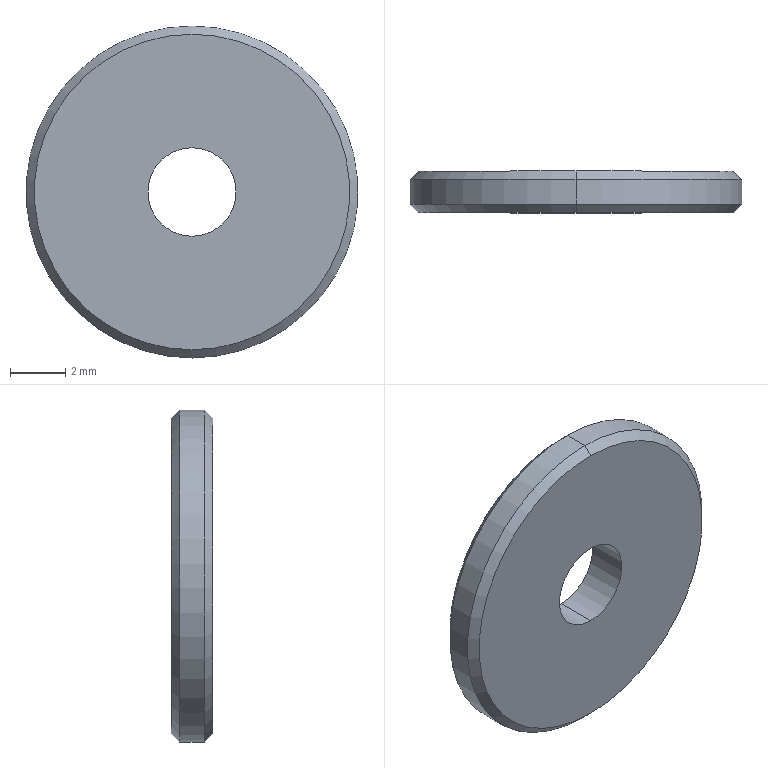Part | SolidWorks | features Chamfer 1, Extrusion 1 | 1 solid | 10 faces | box 12 x 1.5 x 12 mm | volume 154.246 mm3 | cone 4 | cylinder 4 | plane 2 | commonest cylinder face diameters 3.2 x2 12 x2
STEP:
#1=CARTESIAN_POINT('',(0.,1.5,5.7));
#2=VERTEX_POINT('',#1);
#3=CARTESIAN_POINT('',(0.,1.5,-5.7));
#4=VERTEX_POINT('',#3);
#5=CARTESIAN_POINT('',(0.,1.5,0.));
#6=DIRECTION('',(0.,1.,0.));
#7=DIRECTION('',(0.,0.,1.));
#8=AXIS2_PLACEMENT_3D('',#5,#6,#7);
#9=CIRCLE('',#8,5.7);
#10=EDGE_CURVE('',#2,#4,#9,.T.);
#11=ORIENTED_EDGE('',*,*,#10,.F.);
#12=CARTESIAN_POINT('',(0.,1.2,6.));
#13=VERTEX_POINT('',#12);
#14=CARTESIAN_POINT('',(0.,1.5,5.7));
#15=DIRECTION('',(0.,-0.7071,0.7071));
#16=VECTOR('',#15,1000.);
#17=LINE('',#14,#16);
#18=EDGE_CURVE('',#2,#13,#17,.T.);
#19=ORIENTED_EDGE('',*,*,#18,.T.);
#20=CARTESIAN_POINT('',(0.,1.2,-6.));
#21=VERTEX_POINT('',#20);
#22=CARTESIAN_POINT('',(0.,1.2,0.));
#23=DIRECTION('',(0.,-1.,0.));
#24=DIRECTION('',(0.,0.,1.));
#25=AXIS2_PLACEMENT_3D('',#22,#23,#24);
#26=CIRCLE('',#25,6.);
#27=EDGE_CURVE('',#21,#13,#26,.T.);
#28=ORIENTED_EDGE('',*,*,#27,.F.);
#29=CARTESIAN_POINT('',(0.,1.5,-5.7));
#30=DIRECTION('',(0.,-0.7071,-0.7071));
#31=VECTOR('',#30,1000.);
#32=LINE('',#29,#31);
#33=EDGE_CURVE('',#4,#21,#32,.T.);
#34=ORIENTED_EDGE('',*,*,#33,.F.);
#35=EDGE_LOOP('',(#11,#19,#28,#34));
#36=FACE_OUTER_BOUND('',#35,.T.);
#37=CARTESIAN_POINT('',(0.,1.5,0.));
#38=DIRECTION('',(0.,-1.,0.));
#39=DIRECTION('',(0.,0.,-1.));
#40=AXIS2_PLACEMENT_3D('',#37,#38,#39);
#41=CONICAL_SURFACE('',#40,5.7,0.7854);
#42=ADVANCED_FACE('',(#36),#41,.T.);
#43=CARTESIAN_POINT('',(0.,0.,-5.7));
#44=VERTEX_POINT('',#43);
#45=CARTESIAN_POINT('',(0.,0.,5.7));
#46=VERTEX_POINT('',#45);
#47=CARTESIAN_POINT('',(0.,0.,0.));
#48=DIRECTION('',(0.,-1.,0.));
#49=DIRECTION('',(0.,0.,1.));
#50=AXIS2_PLACEMENT_3D('',#47,#48,#49);
#51=CIRCLE('',#50,5.7);
#52=EDGE_CURVE('',#44,#46,#51,.T.);
#53=ORIENTED_EDGE('',*,*,#52,.F.);
#54=CARTESIAN_POINT('',(0.,0.3,-6.));
#55=VERTEX_POINT('',#54);
#56=CARTESIAN_POINT('',(0.,0.3,-6.));
#57=DIRECTION('',(0.,0.7071,-0.7071));
#58=VECTOR('',#57,1000.);
#59=LINE('',#56,#58);
#60=EDGE_CURVE('',#44,#55,#59,.T.);
#61=ORIENTED_EDGE('',*,*,#60,.T.);
#62=CARTESIAN_POINT('',(0.,0.3,6.));
#63=VERTEX_POINT('',#62);
#64=CARTESIAN_POINT('',(0.,0.3,0.));
#65=DIRECTION('',(0.,1.,0.));
#66=DIRECTION('',(0.,0.,1.));
#67=AXIS2_PLACEMENT_3D('',#64,#65,#66);
#68=CIRCLE('',#67,6.);
#69=EDGE_CURVE('',#63,#55,#68,.T.);
#70=ORIENTED_EDGE('',*,*,#69,.F.);
#71=CARTESIAN_POINT('',(0.,0.3,6.));
#72=DIRECTION('',(0.,0.7071,0.7071));
#73=VECTOR('',#72,1000.);
#74=LINE('',#71,#73);
#75=EDGE_CURVE('',#46,#63,#74,.T.);
#76=ORIENTED_EDGE('',*,*,#75,.F.);
#77=EDGE_LOOP('',(#53,#61,#70,#76));
#78=FACE_OUTER_BOUND('',#77,.T.);
#79=CARTESIAN_POINT('',(0.,0.3,0.));
#80=DIRECTION('',(0.,1.,0.));
#81=DIRECTION('',(0.,0.,1.));
#82=AXIS2_PLACEMENT_3D('',#79,#80,#81);
#83=CONICAL_SURFACE('',#82,6.,0.7854);
#84=ADVANCED_FACE('',(#78),#83,.T.);
#85=CARTESIAN_POINT('',(0.,1.5,-1.6));
#86=VERTEX_POINT('',#85);
#87=CARTESIAN_POINT('',(0.,1.5,1.6));
#88=VERTEX_POINT('',#87);
#89=CARTESIAN_POINT('',(0.,1.5,0.));
#90=DIRECTION('',(0.,1.,0.));
#91=DIRECTION('',(0.,0.,1.));
#92=AXIS2_PLACEMENT_3D('',#89,#90,#91);
#93=CIRCLE('',#92,1.6);
#94=EDGE_CURVE('',#86,#88,#93,.T.);
#95=ORIENTED_EDGE('',*,*,#94,.T.);
#96=CARTESIAN_POINT('',(0.,0.,1.6));
#97=VERTEX_POINT('',#96);
#98=CARTESIAN_POINT('',(0.,1.5,1.6));
#99=DIRECTION('',(0.,-1.,0.));
#100=VECTOR('',#99,1000.);
#101=LINE('',#98,#100);
#102=EDGE_CURVE('',#88,#97,#101,.T.);
#103=ORIENTED_EDGE('',*,*,#102,.T.);
#104=CARTESIAN_POINT('',(0.,0.,-1.6));
#105=VERTEX_POINT('',#104);
#106=CARTESIAN_POINT('',(0.,0.,0.));
#107=DIRECTION('',(0.,1.,0.));
#108=DIRECTION('',(0.,0.,1.));
#109=AXIS2_PLACEMENT_3D('',#106,#107,#108);
#110=CIRCLE('',#109,1.6);
#111=EDGE_CURVE('',#105,#97,#110,.T.);
#112=ORIENTED_EDGE('',*,*,#111,.F.);
#113=CARTESIAN_POINT('',(0.,1.5,-1.6));
#114=DIRECTION('',(0.,-1.,0.));
#115=VECTOR('',#114,1000.);
#116=LINE('',#113,#115);
#117=EDGE_CURVE('',#86,#105,#116,.T.);
#118=ORIENTED_EDGE('',*,*,#117,.F.);
#119=EDGE_LOOP('',(#95,#103,#112,#118));
#120=FACE_OUTER_BOUND('',#119,.T.);
#121=CARTESIAN_POINT('',(0.,1.5,0.));
#122=DIRECTION('',(0.,-1.,0.));
#123=DIRECTION('',(0.,0.,-1.));
#124=AXIS2_PLACEMENT_3D('',#121,#122,#123);
#125=CYLINDRICAL_SURFACE('',#124,1.6);
#126=ADVANCED_FACE('',(#120),#125,.F.);
#127=ORIENTED_EDGE('',*,*,#27,.T.);
#128=CARTESIAN_POINT('',(0.,1.5,6.));
#129=DIRECTION('',(0.,-1.,0.));
#130=VECTOR('',#129,1000.);
#131=LINE('',#128,#130);
#132=EDGE_CURVE('',#13,#63,#131,.T.);
#133=ORIENTED_EDGE('',*,*,#132,.T.);
#134=ORIENTED_EDGE('',*,*,#69,.T.);
#135=CARTESIAN_POINT('',(0.,1.5,-6.));
#136=DIRECTION('',(0.,-1.,0.));
#137=VECTOR('',#136,1000.);
#138=LINE('',#135,#137);
#139=EDGE_CURVE('',#21,#55,#138,.T.);
#140=ORIENTED_EDGE('',*,*,#139,.F.);
#141=EDGE_LOOP('',(#127,#133,#134,#140));
#142=FACE_OUTER_BOUND('',#141,.T.);
#143=CARTESIAN_POINT('',(0.,1.5,0.));
#144=DIRECTION('',(0.,-1.,0.));
#145=DIRECTION('',(0.,0.,-1.));
#146=AXIS2_PLACEMENT_3D('',#143,#144,#145);
#147=CYLINDRICAL_SURFACE('',#146,6.);
#148=ADVANCED_FACE('',(#142),#147,.T.);
#149=CARTESIAN_POINT('',(0.,1.5,0.));
#150=DIRECTION('',(0.,1.,0.));
#151=DIRECTION('',(0.,0.,1.));
#152=AXIS2_PLACEMENT_3D('',#149,#150,#151);
#153=CIRCLE('',#152,5.7);
#154=EDGE_CURVE('',#4,#2,#153,.T.);
#155=ORIENTED_EDGE('',*,*,#154,.T.);
#156=ORIENTED_EDGE('',*,*,#10,.T.);
#157=EDGE_LOOP('',(#155,#156));
#158=FACE_OUTER_BOUND('',#157,.T.);
#159=ORIENTED_EDGE('',*,*,#94,.F.);
#160=CARTESIAN_POINT('',(0.,1.5,0.));
#161=DIRECTION('',(0.,1.,0.));
#162=DIRECTION('',(0.,0.,1.));
#163=AXIS2_PLACEMENT_3D('',#160,#161,#162);
#164=CIRCLE('',#163,1.6);
#165=EDGE_CURVE('',#88,#86,#164,.T.);
#166=ORIENTED_EDGE('',*,*,#165,.F.);
#167=EDGE_LOOP('',(#159,#166));
#168=FACE_BOUND('',#167,.T.);
#169=CARTESIAN_POINT('',(0.,1.5,0.));
#170=DIRECTION('',(0.,1.,0.));
#171=DIRECTION('',(0.,0.,1.));
#172=AXIS2_PLACEMENT_3D('',#169,#170,#171);
#173=PLANE('',#172);
#174=ADVANCED_FACE('',(#158,#168),#173,.T.);
#175=CARTESIAN_POINT('',(0.,0.,0.));
#176=DIRECTION('',(0.,-1.,0.));
#177=DIRECTION('',(0.,0.,1.));
#178=AXIS2_PLACEMENT_3D('',#175,#176,#177);
#179=CIRCLE('',#178,5.7);
#180=EDGE_CURVE('',#46,#44,#179,.T.);
#181=ORIENTED_EDGE('',*,*,#180,.T.);
#182=ORIENTED_EDGE('',*,*,#52,.T.);
#183=EDGE_LOOP('',(#181,#182));
#184=FACE_OUTER_BOUND('',#183,.T.);
#185=ORIENTED_EDGE('',*,*,#111,.T.);
#186=CARTESIAN_POINT('',(0.,0.,0.));
#187=DIRECTION('',(0.,1.,0.));
#188=DIRECTION('',(0.,0.,1.));
#189=AXIS2_PLACEMENT_3D('',#186,#187,#188);
#190=CIRCLE('',#189,1.6);
#191=EDGE_CURVE('',#97,#105,#190,.T.);
#192=ORIENTED_EDGE('',*,*,#191,.T.);
#193=EDGE_LOOP('',(#185,#192));
#194=FACE_BOUND('',#193,.T.);
#195=CARTESIAN_POINT('',(0.,0.,0.));
#196=DIRECTION('',(0.,1.,0.));
#197=DIRECTION('',(0.,0.,1.));
#198=AXIS2_PLACEMENT_3D('',#195,#196,#197);
#199=PLANE('',#198);
#200=ADVANCED_FACE('',(#184,#194),#199,.F.);
#201=ORIENTED_EDGE('',*,*,#132,.F.);
#202=CARTESIAN_POINT('',(0.,1.2,0.));
#203=DIRECTION('',(0.,-1.,0.));
#204=DIRECTION('',(0.,0.,1.));
#205=AXIS2_PLACEMENT_3D('',#202,#203,#204);
#206=CIRCLE('',#205,6.);
#207=EDGE_CURVE('',#13,#21,#206,.T.);
#208=ORIENTED_EDGE('',*,*,#207,.T.);
#209=ORIENTED_EDGE('',*,*,#139,.T.);
#210=CARTESIAN_POINT('',(0.,0.3,0.));
#211=DIRECTION('',(0.,1.,0.));
#212=DIRECTION('',(0.,0.,1.));
#213=AXIS2_PLACEMENT_3D('',#210,#211,#212);
#214=CIRCLE('',#213,6.);
#215=EDGE_CURVE('',#55,#63,#214,.T.);
#216=ORIENTED_EDGE('',*,*,#215,.T.);
#217=EDGE_LOOP('',(#201,#208,#209,#216));
#218=FACE_OUTER_BOUND('',#217,.T.);
#219=CARTESIAN_POINT('',(0.,1.5,0.));
#220=DIRECTION('',(0.,-1.,0.));
#221=DIRECTION('',(0.,0.,-1.));
#222=AXIS2_PLACEMENT_3D('',#219,#220,#221);
#223=CYLINDRICAL_SURFACE('',#222,6.);
#224=ADVANCED_FACE('',(#218),#223,.T.);
#225=ORIENTED_EDGE('',*,*,#102,.F.);
#226=ORIENTED_EDGE('',*,*,#165,.T.);
#227=ORIENTED_EDGE('',*,*,#117,.T.);
#228=ORIENTED_EDGE('',*,*,#191,.F.);
#229=EDGE_LOOP('',(#225,#226,#227,#228));
#230=FACE_OUTER_BOUND('',#229,.T.);
#231=CARTESIAN_POINT('',(0.,1.5,0.));
#232=DIRECTION('',(0.,-1.,0.));
#233=DIRECTION('',(0.,0.,-1.));
#234=AXIS2_PLACEMENT_3D('',#231,#232,#233);
#235=CYLINDRICAL_SURFACE('',#234,1.6);
#236=ADVANCED_FACE('',(#230),#235,.F.);
#237=ORIENTED_EDGE('',*,*,#60,.F.);
#238=ORIENTED_EDGE('',*,*,#180,.F.);
#239=ORIENTED_EDGE('',*,*,#75,.T.);
#240=ORIENTED_EDGE('',*,*,#215,.F.);
#241=EDGE_LOOP('',(#237,#238,#239,#240));
#242=FACE_OUTER_BOUND('',#241,.T.);
#243=CARTESIAN_POINT('',(0.,0.3,0.));
#244=DIRECTION('',(0.,1.,0.));
#245=DIRECTION('',(0.,0.,1.));
#246=AXIS2_PLACEMENT_3D('',#243,#244,#245);
#247=CONICAL_SURFACE('',#246,6.,0.7854);
#248=ADVANCED_FACE('',(#242),#247,.T.);
#249=ORIENTED_EDGE('',*,*,#18,.F.);
#250=ORIENTED_EDGE('',*,*,#154,.F.);
#251=ORIENTED_EDGE('',*,*,#33,.T.);
#252=ORIENTED_EDGE('',*,*,#207,.F.);
#253=EDGE_LOOP('',(#249,#250,#251,#252));
#254=FACE_OUTER_BOUND('',#253,.T.);
#255=CARTESIAN_POINT('',(0.,1.5,0.));
#256=DIRECTION('',(0.,-1.,0.));
#257=DIRECTION('',(0.,0.,-1.));
#258=AXIS2_PLACEMENT_3D('',#255,#256,#257);
#259=CONICAL_SURFACE('',#258,5.7,0.7854);
#260=ADVANCED_FACE('',(#254),#259,.T.);
#261=CLOSED_SHELL('',(#42,#84,#126,#148,#174,#200,#224,#236,#248,#260));
#262=MANIFOLD_SOLID_BREP('',#261);
#263=CARTESIAN_POINT('',(0.,0.,0.));
#264=DIRECTION('',(0.,0.,1.));
#265=DIRECTION('',(1.,0.,0.));
#266=AXIS2_PLACEMENT_3D('',#263,#264,#265);
#267=(LENGTH_UNIT()NAMED_UNIT(*)SI_UNIT(.MILLI.,.METRE.));
#268=UNCERTAINTY_MEASURE_WITH_UNIT(LENGTH_MEASURE(0.00001),#267,'','');
#269=(NAMED_UNIT(*)PLANE_ANGLE_UNIT()SI_UNIT($,.RADIAN.));
#270=(NAMED_UNIT(*)SI_UNIT($,.STERADIAN.)SOLID_ANGLE_UNIT());
#271=(GEOMETRIC_REPRESENTATION_CONTEXT(3)GLOBAL_UNCERTAINTY_ASSIGNED_CONTEXT((#268))GLOBAL_UNIT_ASSIGNED_CONTEXT((#267,#269,#270))REPRESENTATION_CONTEXT('',''));
#272=ADVANCED_BREP_SHAPE_REPRESENTATION('',(#262,#266),#271);